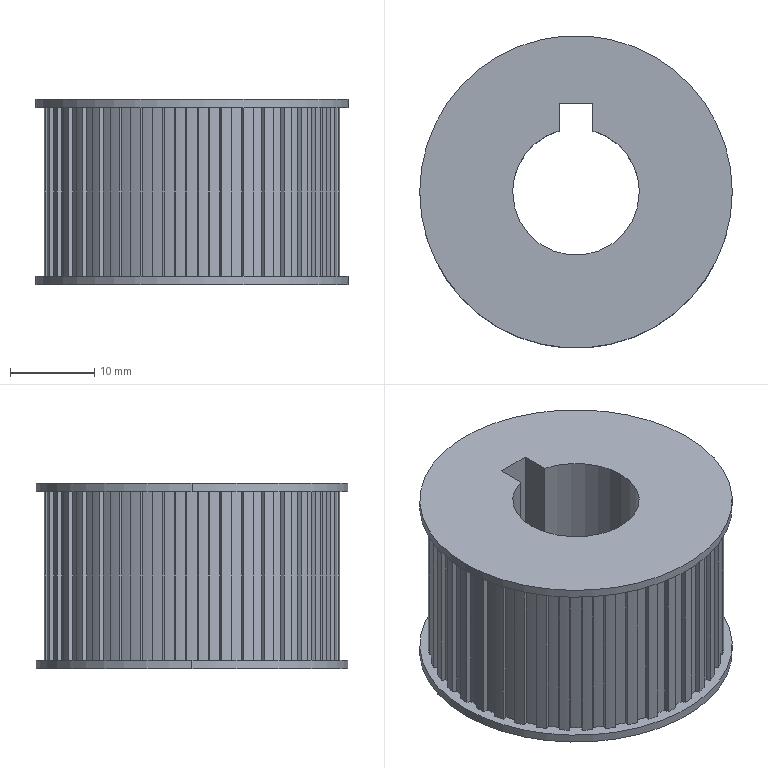Part | STEP file | Timing pulley | 1 solid | 175 faces | box 37 x 37 x 22 mm | volume 16663 mm3 | cylinder 88 | plane 87 | commonest cylinder face diameters 34 x41 35 x40 37 x4 15 x3